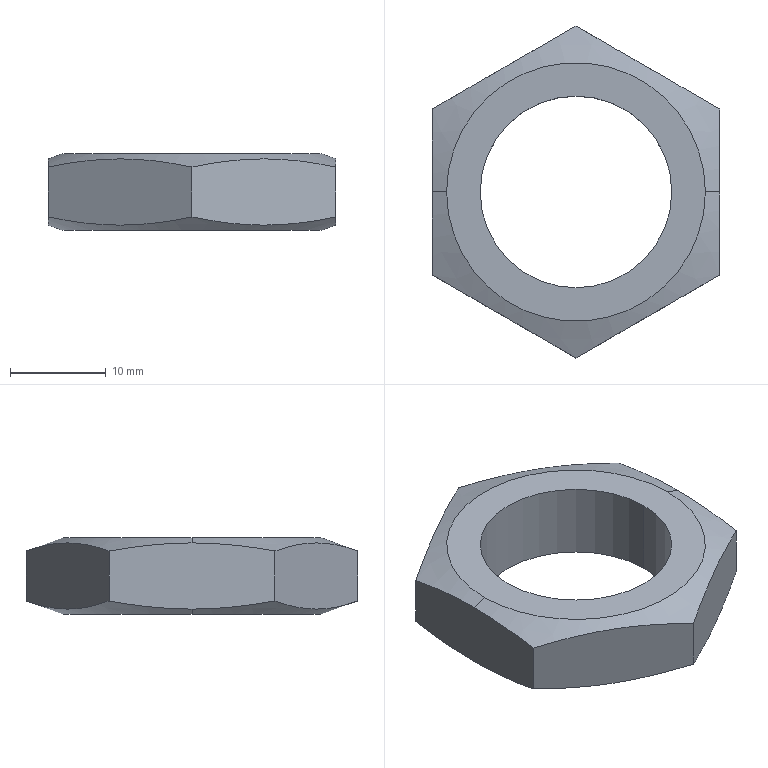Part | SolidWorks | features Extrusion 1, ICE 1, MirrorPattern 1, RefAxis 1, RevCut 1 | 1 solid | 14 faces | box 30 x 34.641 x 8 mm | volume 3531 mm3 | plane 8 | cone 4 | cylinder 2 | commonest cylinder face diameters 20 x2
STEP:
#1=CARTESIAN_POINT('',(-10.,0.,0.));
#2=VERTEX_POINT('',#1);
#3=CARTESIAN_POINT('',(10.,0.,0.));
#4=VERTEX_POINT('',#3);
#5=CARTESIAN_POINT('',(0.,0.,0.));
#6=DIRECTION('',(0.,0.,1.));
#7=DIRECTION('',(1.,0.,0.));
#8=AXIS2_PLACEMENT_3D('',#5,#6,#7);
#9=CIRCLE('',#8,10.);
#10=EDGE_CURVE('',#2,#4,#9,.T.);
#11=ORIENTED_EDGE('',*,*,#10,.F.);
#12=CARTESIAN_POINT('',(-10.,0.,8.));
#13=VERTEX_POINT('',#12);
#14=CARTESIAN_POINT('',(-10.,0.,0.));
#15=DIRECTION('',(0.,0.,1.));
#16=VECTOR('',#15,1000.);
#17=LINE('',#14,#16);
#18=EDGE_CURVE('',#2,#13,#17,.T.);
#19=ORIENTED_EDGE('',*,*,#18,.T.);
#20=CARTESIAN_POINT('',(10.,0.,8.));
#21=VERTEX_POINT('',#20);
#22=CARTESIAN_POINT('',(0.,0.,8.));
#23=DIRECTION('',(0.,0.,1.));
#24=DIRECTION('',(1.,0.,0.));
#25=AXIS2_PLACEMENT_3D('',#22,#23,#24);
#26=CIRCLE('',#25,10.);
#27=EDGE_CURVE('',#13,#21,#26,.T.);
#28=ORIENTED_EDGE('',*,*,#27,.T.);
#29=CARTESIAN_POINT('',(10.,0.,0.));
#30=DIRECTION('',(0.,0.,1.));
#31=VECTOR('',#30,1000.);
#32=LINE('',#29,#31);
#33=EDGE_CURVE('',#4,#21,#32,.T.);
#34=ORIENTED_EDGE('',*,*,#33,.F.);
#35=EDGE_LOOP('',(#11,#19,#28,#34));
#36=FACE_OUTER_BOUND('',#35,.T.);
#37=CARTESIAN_POINT('',(0.,0.,0.));
#38=DIRECTION('',(0.,0.,1.));
#39=DIRECTION('',(1.,0.,0.));
#40=AXIS2_PLACEMENT_3D('',#37,#38,#39);
#41=CYLINDRICAL_SURFACE('',#40,10.);
#42=ADVANCED_FACE('',(#36),#41,.F.);
#43=CARTESIAN_POINT('',(-13.5,0.,0.));
#44=VERTEX_POINT('',#43);
#45=CARTESIAN_POINT('',(13.5,0.,0.));
#46=VERTEX_POINT('',#45);
#47=CARTESIAN_POINT('',(0.,0.,0.));
#48=DIRECTION('',(0.,0.,1.));
#49=DIRECTION('',(1.,0.,0.));
#50=AXIS2_PLACEMENT_3D('',#47,#48,#49);
#51=CIRCLE('',#50,13.5);
#52=EDGE_CURVE('',#44,#46,#51,.T.);
#53=ORIENTED_EDGE('',*,*,#52,.T.);
#54=CARTESIAN_POINT('',(15.,0.,0.546));
#55=VERTEX_POINT('',#54);
#56=CARTESIAN_POINT('',(17.321,0.,1.391));
#57=DIRECTION('',(0.9397,0.,0.342));
#58=VECTOR('',#57,1000.);
#59=LINE('',#56,#58);
#60=EDGE_CURVE('',#46,#55,#59,.T.);
#61=ORIENTED_EDGE('',*,*,#60,.T.);
#62=CARTESIAN_POINT('',(15.,-8.66,1.391));
#63=VERTEX_POINT('',#62);
#64=CARTESIAN_POINT('',(15.,-8.66,1.391));
#65=CARTESIAN_POINT('',(15.,-7.226,1.13));
#66=CARTESIAN_POINT('',(15.,-5.777,0.915));
#67=CARTESIAN_POINT('',(15.,-2.886,0.6231));
#68=CARTESIAN_POINT('',(15.,-1.442,0.546));
#69=CARTESIAN_POINT('',(15.,0.,0.546));
#70=B_SPLINE_CURVE_WITH_KNOTS('',3,(#64,#65,#66,#67,#68,#69),.UNSPECIFIED.,.F.,.F.,(4,2,4),(0.01468,0.01904,0.02341),.UNSPECIFIED.);
#71=EDGE_CURVE('',#63,#55,#70,.T.);
#72=ORIENTED_EDGE('',*,*,#71,.F.);
#73=CARTESIAN_POINT('',(0.,-17.321,1.391));
#74=VERTEX_POINT('',#73);
#75=CARTESIAN_POINT('',(0.,-17.321,1.391));
#76=CARTESIAN_POINT('',(1.25,-16.599,1.128));
#77=CARTESIAN_POINT('',(2.5,-15.877,0.9146));
#78=CARTESIAN_POINT('',(5.,-14.434,0.6232));
#79=CARTESIAN_POINT('',(7.5,-12.99,0.4687));
#80=CARTESIAN_POINT('',(10.,-11.547,0.6232));
#81=CARTESIAN_POINT('',(12.5,-10.104,0.9146));
#82=CARTESIAN_POINT('',(13.75,-9.382,1.128));
#83=CARTESIAN_POINT('',(15.,-8.66,1.391));
#84=B_SPLINE_CURVE_WITH_KNOTS('',3,(#75,#76,#77,#78,#79,#80,#81,#82,#83),.UNSPECIFIED.,.F.,.F.,(4,2,1,2,4),(0.000000231,0.00433,0.00866,0.01299,0.01732),.UNSPECIFIED.);
#85=EDGE_CURVE('',#74,#63,#84,.T.);
#86=ORIENTED_EDGE('',*,*,#85,.F.);
#87=CARTESIAN_POINT('',(-15.,-8.66,1.391));
#88=VERTEX_POINT('',#87);
#89=CARTESIAN_POINT('',(-15.,-8.66,1.391));
#90=CARTESIAN_POINT('',(-13.75,-9.382,1.128));
#91=CARTESIAN_POINT('',(-12.5,-10.104,0.9146));
#92=CARTESIAN_POINT('',(-10.,-11.547,0.6232));
#93=CARTESIAN_POINT('',(-7.5,-12.99,0.4687));
#94=CARTESIAN_POINT('',(-5.,-14.434,0.6232));
#95=CARTESIAN_POINT('',(-2.5,-15.877,0.9146));
#96=CARTESIAN_POINT('',(-1.25,-16.599,1.128));
#97=CARTESIAN_POINT('',(0.,-17.321,1.391));
#98=B_SPLINE_CURVE_WITH_KNOTS('',3,(#89,#90,#91,#92,#93,#94,#95,#96,#97),.UNSPECIFIED.,.F.,.F.,(4,2,1,2,4),(0.000000231,0.00433,0.00866,0.01299,0.01732),.UNSPECIFIED.);
#99=EDGE_CURVE('',#88,#74,#98,.T.);
#100=ORIENTED_EDGE('',*,*,#99,.F.);
#101=CARTESIAN_POINT('',(-15.,0.,0.546));
#102=VERTEX_POINT('',#101);
#103=CARTESIAN_POINT('',(-15.,0.,0.546));
#104=CARTESIAN_POINT('',(-15.,-1.442,0.546));
#105=CARTESIAN_POINT('',(-15.,-2.886,0.6231));
#106=CARTESIAN_POINT('',(-15.,-5.777,0.915));
#107=CARTESIAN_POINT('',(-15.,-7.226,1.13));
#108=CARTESIAN_POINT('',(-15.,-8.66,1.391));
#109=B_SPLINE_CURVE_WITH_KNOTS('',3,(#103,#104,#105,#106,#107,#108),.UNSPECIFIED.,.F.,.F.,(4,2,4),(0.04016,0.04451,0.04886),.UNSPECIFIED.);
#110=EDGE_CURVE('',#102,#88,#109,.T.);
#111=ORIENTED_EDGE('',*,*,#110,.F.);
#112=CARTESIAN_POINT('',(-17.321,0.,1.391));
#113=DIRECTION('',(-0.9397,0.,0.342));
#114=VECTOR('',#113,1000.);
#115=LINE('',#112,#114);
#116=EDGE_CURVE('',#44,#102,#115,.T.);
#117=ORIENTED_EDGE('',*,*,#116,.F.);
#118=EDGE_LOOP('',(#53,#61,#72,#86,#100,#111,#117));
#119=FACE_OUTER_BOUND('',#118,.T.);
#120=CARTESIAN_POINT('',(0.,0.,1.391));
#121=DIRECTION('',(0.,0.,1.));
#122=DIRECTION('',(-1.,0.,0.));
#123=AXIS2_PLACEMENT_3D('',#120,#121,#122);
#124=CONICAL_SURFACE('',#123,17.321,1.222);
#125=ADVANCED_FACE('',(#119),#124,.T.);
#126=CARTESIAN_POINT('',(13.5,0.,8.));
#127=VERTEX_POINT('',#126);
#128=CARTESIAN_POINT('',(-13.5,0.,8.));
#129=VERTEX_POINT('',#128);
#130=CARTESIAN_POINT('',(0.,0.,8.));
#131=DIRECTION('',(0.,0.,1.));
#132=DIRECTION('',(1.,0.,0.));
#133=AXIS2_PLACEMENT_3D('',#130,#131,#132);
#134=CIRCLE('',#133,13.5);
#135=EDGE_CURVE('',#127,#129,#134,.T.);
#136=ORIENTED_EDGE('',*,*,#135,.F.);
#137=CARTESIAN_POINT('',(15.,0.,7.454));
#138=VERTEX_POINT('',#137);
#139=CARTESIAN_POINT('',(17.321,0.,6.609));
#140=DIRECTION('',(0.9397,0.,-0.342));
#141=VECTOR('',#140,1000.);
#142=LINE('',#139,#141);
#143=EDGE_CURVE('',#127,#138,#142,.T.);
#144=ORIENTED_EDGE('',*,*,#143,.T.);
#145=CARTESIAN_POINT('',(15.,8.66,6.609));
#146=VERTEX_POINT('',#145);
#147=CARTESIAN_POINT('',(15.,8.66,6.609));
#148=CARTESIAN_POINT('',(15.,7.221,6.871));
#149=CARTESIAN_POINT('',(15.,5.778,7.085));
#150=CARTESIAN_POINT('',(15.,2.891,7.377));
#151=CARTESIAN_POINT('',(15.,1.446,7.454));
#152=CARTESIAN_POINT('',(15.,0.,7.454));
#153=B_SPLINE_CURVE_WITH_KNOTS('',3,(#147,#148,#149,#150,#151,#152),.UNSPECIFIED.,.F.,.F.,(4,2,4),(0.03143,0.03579,0.04016),.UNSPECIFIED.);
#154=EDGE_CURVE('',#146,#138,#153,.T.);
#155=ORIENTED_EDGE('',*,*,#154,.F.);
#156=CARTESIAN_POINT('',(0.,17.321,6.609));
#157=VERTEX_POINT('',#156);
#158=CARTESIAN_POINT('',(0.,17.321,6.609));
#159=CARTESIAN_POINT('',(1.25,16.599,6.872));
#160=CARTESIAN_POINT('',(2.5,15.877,7.085));
#161=CARTESIAN_POINT('',(5.,14.434,7.377));
#162=CARTESIAN_POINT('',(7.5,12.99,7.531));
#163=CARTESIAN_POINT('',(10.,11.547,7.377));
#164=CARTESIAN_POINT('',(12.5,10.104,7.085));
#165=CARTESIAN_POINT('',(13.75,9.382,6.872));
#166=CARTESIAN_POINT('',(15.,8.66,6.609));
#167=B_SPLINE_CURVE_WITH_KNOTS('',3,(#158,#159,#160,#161,#162,#163,#164,#165,#166),.UNSPECIFIED.,.F.,.F.,(4,2,1,2,4),(0.000000231,0.00433,0.00866,0.01299,0.01732),.UNSPECIFIED.);
#168=EDGE_CURVE('',#157,#146,#167,.T.);
#169=ORIENTED_EDGE('',*,*,#168,.F.);
#170=CARTESIAN_POINT('',(-15.,8.66,6.609));
#171=VERTEX_POINT('',#170);
#172=CARTESIAN_POINT('',(-15.,8.66,6.609));
#173=CARTESIAN_POINT('',(-13.75,9.382,6.872));
#174=CARTESIAN_POINT('',(-12.5,10.104,7.085));
#175=CARTESIAN_POINT('',(-10.,11.547,7.377));
#176=CARTESIAN_POINT('',(-7.5,12.99,7.531));
#177=CARTESIAN_POINT('',(-5.,14.434,7.377));
#178=CARTESIAN_POINT('',(-2.5,15.877,7.085));
#179=CARTESIAN_POINT('',(-1.25,16.599,6.872));
#180=CARTESIAN_POINT('',(0.,17.321,6.609));
#181=B_SPLINE_CURVE_WITH_KNOTS('',3,(#172,#173,#174,#175,#176,#177,#178,#179,#180),.UNSPECIFIED.,.F.,.F.,(4,2,1,2,4),(0.000000231,0.00433,0.00866,0.01299,0.01732),.UNSPECIFIED.);
#182=EDGE_CURVE('',#171,#157,#181,.T.);
#183=ORIENTED_EDGE('',*,*,#182,.F.);
#184=CARTESIAN_POINT('',(-15.,0.,7.454));
#185=VERTEX_POINT('',#184);
#186=CARTESIAN_POINT('',(-15.,0.,7.454));
#187=CARTESIAN_POINT('',(-15.,1.446,7.454));
#188=CARTESIAN_POINT('',(-15.,2.891,7.377));
#189=CARTESIAN_POINT('',(-15.,5.778,7.085));
#190=CARTESIAN_POINT('',(-15.,7.221,6.871));
#191=CARTESIAN_POINT('',(-15.,8.66,6.609));
#192=B_SPLINE_CURVE_WITH_KNOTS('',3,(#186,#187,#188,#189,#190,#191),.UNSPECIFIED.,.F.,.F.,(4,2,4),(0.02341,0.02778,0.03216),.UNSPECIFIED.);
#193=EDGE_CURVE('',#185,#171,#192,.T.);
#194=ORIENTED_EDGE('',*,*,#193,.F.);
#195=CARTESIAN_POINT('',(-17.321,0.,6.609));
#196=DIRECTION('',(-0.9397,0.,-0.342));
#197=VECTOR('',#196,1000.);
#198=LINE('',#195,#197);
#199=EDGE_CURVE('',#129,#185,#198,.T.);
#200=ORIENTED_EDGE('',*,*,#199,.F.);
#201=EDGE_LOOP('',(#136,#144,#155,#169,#183,#194,#200));
#202=FACE_OUTER_BOUND('',#201,.T.);
#203=CARTESIAN_POINT('',(0.,0.,6.609));
#204=DIRECTION('',(0.,0.,-1.));
#205=DIRECTION('',(-1.,0.,0.));
#206=AXIS2_PLACEMENT_3D('',#203,#204,#205);
#207=CONICAL_SURFACE('',#206,17.321,1.222);
#208=ADVANCED_FACE('',(#202),#207,.T.);
#209=CARTESIAN_POINT('',(15.,8.66,1.391));
#210=VERTEX_POINT('',#209);
#211=CARTESIAN_POINT('',(15.,8.66,8.));
#212=DIRECTION('',(0.,0.,-1.));
#213=VECTOR('',#212,1000.);
#214=LINE('',#211,#213);
#215=EDGE_CURVE('',#146,#210,#214,.T.);
#216=ORIENTED_EDGE('',*,*,#215,.T.);
#217=CARTESIAN_POINT('',(0.,17.321,1.391));
#218=VERTEX_POINT('',#217);
#219=CARTESIAN_POINT('',(15.,8.66,1.391));
#220=CARTESIAN_POINT('',(13.75,9.382,1.128));
#221=CARTESIAN_POINT('',(12.5,10.104,0.9146));
#222=CARTESIAN_POINT('',(10.,11.547,0.6232));
#223=CARTESIAN_POINT('',(7.5,12.99,0.4687));
#224=CARTESIAN_POINT('',(5.,14.434,0.6232));
#225=CARTESIAN_POINT('',(2.5,15.877,0.9146));
#226=CARTESIAN_POINT('',(1.25,16.599,1.128));
#227=CARTESIAN_POINT('',(0.,17.321,1.391));
#228=B_SPLINE_CURVE_WITH_KNOTS('',3,(#219,#220,#221,#222,#223,#224,#225,#226,#227),.UNSPECIFIED.,.F.,.F.,(4,2,1,2,4),(0.000000231,0.00433,0.00866,0.01299,0.01732),.UNSPECIFIED.);
#229=EDGE_CURVE('',#210,#218,#228,.T.);
#230=ORIENTED_EDGE('',*,*,#229,.T.);
#231=CARTESIAN_POINT('',(0.,17.321,8.));
#232=DIRECTION('',(0.,0.,-1.));
#233=VECTOR('',#232,1000.);
#234=LINE('',#231,#233);
#235=EDGE_CURVE('',#157,#218,#234,.T.);
#236=ORIENTED_EDGE('',*,*,#235,.F.);
#237=ORIENTED_EDGE('',*,*,#168,.T.);
#238=EDGE_LOOP('',(#216,#230,#236,#237));
#239=FACE_OUTER_BOUND('',#238,.T.);
#240=CARTESIAN_POINT('',(15.,8.66,8.));
#241=DIRECTION('',(-0.5,-0.866,0.));
#242=DIRECTION('',(0.866,-0.5,0.));
#243=AXIS2_PLACEMENT_3D('',#240,#241,#242);
#244=PLANE('',#243);
#245=ADVANCED_FACE('',(#239),#244,.F.);
#246=ORIENTED_EDGE('',*,*,#235,.T.);
#247=CARTESIAN_POINT('',(-15.,8.66,1.391));
#248=VERTEX_POINT('',#247);
#249=CARTESIAN_POINT('',(0.,17.321,1.391));
#250=CARTESIAN_POINT('',(-1.25,16.599,1.128));
#251=CARTESIAN_POINT('',(-2.5,15.877,0.9146));
#252=CARTESIAN_POINT('',(-5.,14.434,0.6232));
#253=CARTESIAN_POINT('',(-7.5,12.99,0.4687));
#254=CARTESIAN_POINT('',(-10.,11.547,0.6232));
#255=CARTESIAN_POINT('',(-12.5,10.104,0.9146));
#256=CARTESIAN_POINT('',(-13.75,9.382,1.128));
#257=CARTESIAN_POINT('',(-15.,8.66,1.391));
#258=B_SPLINE_CURVE_WITH_KNOTS('',3,(#249,#250,#251,#252,#253,#254,#255,#256,#257),.UNSPECIFIED.,.F.,.F.,(4,2,1,2,4),(0.000000231,0.00433,0.00866,0.01299,0.01732),.UNSPECIFIED.);
#259=EDGE_CURVE('',#218,#248,#258,.T.);
#260=ORIENTED_EDGE('',*,*,#259,.T.);
#261=CARTESIAN_POINT('',(-15.,8.66,8.));
#262=DIRECTION('',(0.,0.,-1.));
#263=VECTOR('',#262,1000.);
#264=LINE('',#261,#263);
#265=EDGE_CURVE('',#171,#248,#264,.T.);
#266=ORIENTED_EDGE('',*,*,#265,.F.);
#267=ORIENTED_EDGE('',*,*,#182,.T.);
#268=EDGE_LOOP('',(#246,#260,#266,#267));
#269=FACE_OUTER_BOUND('',#268,.T.);
#270=CARTESIAN_POINT('',(0.,17.321,8.));
#271=DIRECTION('',(0.5,-0.866,0.));
#272=DIRECTION('',(0.866,0.5,0.));
#273=AXIS2_PLACEMENT_3D('',#270,#271,#272);
#274=PLANE('',#273);
#275=ADVANCED_FACE('',(#269),#274,.F.);
#276=ORIENTED_EDGE('',*,*,#265,.T.);
#277=CARTESIAN_POINT('',(-15.,8.66,1.391));
#278=CARTESIAN_POINT('',(-15.,7.221,1.129));
#279=CARTESIAN_POINT('',(-15.,5.778,0.9152));
#280=CARTESIAN_POINT('',(-15.,2.891,0.6235));
#281=CARTESIAN_POINT('',(-15.,1.446,0.546));
#282=CARTESIAN_POINT('',(-15.,0.,0.546));
#283=B_SPLINE_CURVE_WITH_KNOTS('',3,(#277,#278,#279,#280,#281,#282),.UNSPECIFIED.,.F.,.F.,(4,2,4),(0.03143,0.03579,0.04016),.UNSPECIFIED.);
#284=EDGE_CURVE('',#248,#102,#283,.T.);
#285=ORIENTED_EDGE('',*,*,#284,.T.);
#286=ORIENTED_EDGE('',*,*,#110,.T.);
#287=CARTESIAN_POINT('',(-15.,-8.66,6.609));
#288=VERTEX_POINT('',#287);
#289=CARTESIAN_POINT('',(-15.,-8.66,8.));
#290=DIRECTION('',(0.,0.,-1.));
#291=VECTOR('',#290,1000.);
#292=LINE('',#289,#291);
#293=EDGE_CURVE('',#288,#88,#292,.T.);
#294=ORIENTED_EDGE('',*,*,#293,.F.);
#295=CARTESIAN_POINT('',(-15.,-8.66,6.609));
#296=CARTESIAN_POINT('',(-15.,-7.226,6.87));
#297=CARTESIAN_POINT('',(-15.,-5.777,7.085));
#298=CARTESIAN_POINT('',(-15.,-2.886,7.377));
#299=CARTESIAN_POINT('',(-15.,-1.442,7.454));
#300=CARTESIAN_POINT('',(-15.,0.,7.454));
#301=B_SPLINE_CURVE_WITH_KNOTS('',3,(#295,#296,#297,#298,#299,#300),.UNSPECIFIED.,.F.,.F.,(4,2,4),(0.01468,0.01904,0.02341),.UNSPECIFIED.);
#302=EDGE_CURVE('',#288,#185,#301,.T.);
#303=ORIENTED_EDGE('',*,*,#302,.T.);
#304=ORIENTED_EDGE('',*,*,#193,.T.);
#305=EDGE_LOOP('',(#276,#285,#286,#294,#303,#304));
#306=FACE_OUTER_BOUND('',#305,.T.);
#307=CARTESIAN_POINT('',(-15.,8.66,8.));
#308=DIRECTION('',(1.,0.,0.));
#309=DIRECTION('',(0.,0.,-1.));
#310=AXIS2_PLACEMENT_3D('',#307,#308,#309);
#311=PLANE('',#310);
#312=ADVANCED_FACE('',(#306),#311,.F.);
#313=ORIENTED_EDGE('',*,*,#293,.T.);
#314=ORIENTED_EDGE('',*,*,#99,.T.);
#315=CARTESIAN_POINT('',(0.,-17.321,6.609));
#316=VERTEX_POINT('',#315);
#317=CARTESIAN_POINT('',(0.,-17.321,8.));
#318=DIRECTION('',(0.,0.,-1.));
#319=VECTOR('',#318,1000.);
#320=LINE('',#317,#319);
#321=EDGE_CURVE('',#316,#74,#320,.T.);
#322=ORIENTED_EDGE('',*,*,#321,.F.);
#323=CARTESIAN_POINT('',(0.,-17.321,6.609));
#324=CARTESIAN_POINT('',(-1.25,-16.599,6.872));
#325=CARTESIAN_POINT('',(-2.5,-15.877,7.085));
#326=CARTESIAN_POINT('',(-5.,-14.434,7.377));
#327=CARTESIAN_POINT('',(-7.5,-12.99,7.531));
#328=CARTESIAN_POINT('',(-10.,-11.547,7.377));
#329=CARTESIAN_POINT('',(-12.5,-10.104,7.085));
#330=CARTESIAN_POINT('',(-13.75,-9.382,6.872));
#331=CARTESIAN_POINT('',(-15.,-8.66,6.609));
#332=B_SPLINE_CURVE_WITH_KNOTS('',3,(#323,#324,#325,#326,#327,#328,#329,#330,#331),.UNSPECIFIED.,.F.,.F.,(4,2,1,2,4),(0.000000231,0.00433,0.00866,0.01299,0.01732),.UNSPECIFIED.);
#333=EDGE_CURVE('',#316,#288,#332,.T.);
#334=ORIENTED_EDGE('',*,*,#333,.T.);
#335=EDGE_LOOP('',(#313,#314,#322,#334));
#336=FACE_OUTER_BOUND('',#335,.T.);
#337=CARTESIAN_POINT('',(-15.,-8.66,8.));
#338=DIRECTION('',(0.5,0.866,0.));
#339=DIRECTION('',(-0.866,0.5,0.));
#340=AXIS2_PLACEMENT_3D('',#337,#338,#339);
#341=PLANE('',#340);
#342=ADVANCED_FACE('',(#336),#341,.F.);
#343=ORIENTED_EDGE('',*,*,#321,.T.);
#344=ORIENTED_EDGE('',*,*,#85,.T.);
#345=CARTESIAN_POINT('',(15.,-8.66,6.609));
#346=VERTEX_POINT('',#345);
#347=CARTESIAN_POINT('',(15.,-8.66,8.));
#348=DIRECTION('',(0.,0.,-1.));
#349=VECTOR('',#348,1000.);
#350=LINE('',#347,#349);
#351=EDGE_CURVE('',#346,#63,#350,.T.);
#352=ORIENTED_EDGE('',*,*,#351,.F.);
#353=CARTESIAN_POINT('',(15.,-8.66,6.609));
#354=CARTESIAN_POINT('',(13.75,-9.382,6.872));
#355=CARTESIAN_POINT('',(12.5,-10.104,7.085));
#356=CARTESIAN_POINT('',(10.,-11.547,7.377));
#357=CARTESIAN_POINT('',(7.5,-12.99,7.531));
#358=CARTESIAN_POINT('',(5.,-14.434,7.377));
#359=CARTESIAN_POINT('',(2.5,-15.877,7.085));
#360=CARTESIAN_POINT('',(1.25,-16.599,6.872));
#361=CARTESIAN_POINT('',(0.,-17.321,6.609));
#362=B_SPLINE_CURVE_WITH_KNOTS('',3,(#353,#354,#355,#356,#357,#358,#359,#360,#361),.UNSPECIFIED.,.F.,.F.,(4,2,1,2,4),(0.000000231,0.00433,0.00866,0.01299,0.01732),.UNSPECIFIED.);
#363=EDGE_CURVE('',#346,#316,#362,.T.);
#364=ORIENTED_EDGE('',*,*,#363,.T.);
#365=EDGE_LOOP('',(#343,#344,#352,#364));
#366=FACE_OUTER_BOUND('',#365,.T.);
#367=CARTESIAN_POINT('',(0.,-17.321,8.));
#368=DIRECTION('',(-0.5,0.866,0.));
#369=DIRECTION('',(-0.866,-0.5,0.));
#370=AXIS2_PLACEMENT_3D('',#367,#368,#369);
#371=PLANE('',#370);
#372=ADVANCED_FACE('',(#366),#371,.F.);
#373=ORIENTED_EDGE('',*,*,#351,.T.);
#374=ORIENTED_EDGE('',*,*,#71,.T.);
#375=CARTESIAN_POINT('',(15.,0.,0.546));
#376=CARTESIAN_POINT('',(15.,1.446,0.546));
#377=CARTESIAN_POINT('',(15.,2.891,0.6235));
#378=CARTESIAN_POINT('',(15.,5.778,0.9152));
#379=CARTESIAN_POINT('',(15.,7.221,1.129));
#380=CARTESIAN_POINT('',(15.,8.66,1.391));
#381=B_SPLINE_CURVE_WITH_KNOTS('',3,(#375,#376,#377,#378,#379,#380),.UNSPECIFIED.,.F.,.F.,(4,2,4),(0.02341,0.02778,0.03216),.UNSPECIFIED.);
#382=EDGE_CURVE('',#55,#210,#381,.T.);
#383=ORIENTED_EDGE('',*,*,#382,.T.);
#384=ORIENTED_EDGE('',*,*,#215,.F.);
#385=ORIENTED_EDGE('',*,*,#154,.T.);
#386=CARTESIAN_POINT('',(15.,0.,7.454));
#387=CARTESIAN_POINT('',(15.,-1.442,7.454));
#388=CARTESIAN_POINT('',(15.,-2.886,7.377));
#389=CARTESIAN_POINT('',(15.,-5.777,7.085));
#390=CARTESIAN_POINT('',(15.,-7.226,6.87));
#391=CARTESIAN_POINT('',(15.,-8.66,6.609));
#392=B_SPLINE_CURVE_WITH_KNOTS('',3,(#386,#387,#388,#389,#390,#391),.UNSPECIFIED.,.F.,.F.,(4,2,4),(0.04016,0.04451,0.04886),.UNSPECIFIED.);
#393=EDGE_CURVE('',#138,#346,#392,.T.);
#394=ORIENTED_EDGE('',*,*,#393,.T.);
#395=EDGE_LOOP('',(#373,#374,#383,#384,#385,#394));
#396=FACE_OUTER_BOUND('',#395,.T.);
#397=CARTESIAN_POINT('',(15.,-8.66,8.));
#398=DIRECTION('',(-1.,0.,0.));
#399=DIRECTION('',(0.,-1.,0.));
#400=AXIS2_PLACEMENT_3D('',#397,#398,#399);
#401=PLANE('',#400);
#402=ADVANCED_FACE('',(#396),#401,.F.);
#403=ORIENTED_EDGE('',*,*,#143,.F.);
#404=CARTESIAN_POINT('',(0.,0.,8.));
#405=DIRECTION('',(0.,0.,1.));
#406=DIRECTION('',(1.,0.,0.));
#407=AXIS2_PLACEMENT_3D('',#404,#405,#406);
#408=CIRCLE('',#407,13.5);
#409=EDGE_CURVE('',#129,#127,#408,.T.);
#410=ORIENTED_EDGE('',*,*,#409,.F.);
#411=ORIENTED_EDGE('',*,*,#199,.T.);
#412=ORIENTED_EDGE('',*,*,#302,.F.);
#413=ORIENTED_EDGE('',*,*,#333,.F.);
#414=ORIENTED_EDGE('',*,*,#363,.F.);
#415=ORIENTED_EDGE('',*,*,#393,.F.);
#416=EDGE_LOOP('',(#403,#410,#411,#412,#413,#414,#415));
#417=FACE_OUTER_BOUND('',#416,.T.);
#418=CARTESIAN_POINT('',(0.,0.,6.609));
#419=DIRECTION('',(0.,0.,-1.));
#420=DIRECTION('',(-1.,0.,0.));
#421=AXIS2_PLACEMENT_3D('',#418,#419,#420);
#422=CONICAL_SURFACE('',#421,17.321,1.222);
#423=ADVANCED_FACE('',(#417),#422,.T.);
#424=CARTESIAN_POINT('',(0.,0.,8.));
#425=DIRECTION('',(0.,0.,1.));
#426=DIRECTION('',(1.,0.,0.));
#427=AXIS2_PLACEMENT_3D('',#424,#425,#426);
#428=CIRCLE('',#427,10.);
#429=EDGE_CURVE('',#21,#13,#428,.T.);
#430=ORIENTED_EDGE('',*,*,#429,.F.);
#431=ORIENTED_EDGE('',*,*,#27,.F.);
#432=EDGE_LOOP('',(#430,#431));
#433=FACE_BOUND('',#432,.T.);
#434=ORIENTED_EDGE('',*,*,#409,.T.);
#435=ORIENTED_EDGE('',*,*,#135,.T.);
#436=EDGE_LOOP('',(#434,#435));
#437=FACE_OUTER_BOUND('',#436,.T.);
#438=CARTESIAN_POINT('',(0.,0.,8.));
#439=DIRECTION('',(0.,0.,1.));
#440=DIRECTION('',(1.,0.,0.));
#441=AXIS2_PLACEMENT_3D('',#438,#439,#440);
#442=PLANE('',#441);
#443=ADVANCED_FACE('',(#433,#437),#442,.T.);
#444=ORIENTED_EDGE('',*,*,#60,.F.);
#445=CARTESIAN_POINT('',(0.,0.,0.));
#446=DIRECTION('',(0.,0.,1.));
#447=DIRECTION('',(1.,0.,0.));
#448=AXIS2_PLACEMENT_3D('',#445,#446,#447);
#449=CIRCLE('',#448,13.5);
#450=EDGE_CURVE('',#46,#44,#449,.T.);
#451=ORIENTED_EDGE('',*,*,#450,.T.);
#452=ORIENTED_EDGE('',*,*,#116,.T.);
#453=ORIENTED_EDGE('',*,*,#284,.F.);
#454=ORIENTED_EDGE('',*,*,#259,.F.);
#455=ORIENTED_EDGE('',*,*,#229,.F.);
#456=ORIENTED_EDGE('',*,*,#382,.F.);
#457=EDGE_LOOP('',(#444,#451,#452,#453,#454,#455,#456));
#458=FACE_OUTER_BOUND('',#457,.T.);
#459=CARTESIAN_POINT('',(0.,0.,1.391));
#460=DIRECTION('',(0.,0.,1.));
#461=DIRECTION('',(-1.,0.,0.));
#462=AXIS2_PLACEMENT_3D('',#459,#460,#461);
#463=CONICAL_SURFACE('',#462,17.321,1.222);
#464=ADVANCED_FACE('',(#458),#463,.T.);
#465=CARTESIAN_POINT('',(0.,0.,0.));
#466=DIRECTION('',(0.,0.,1.));
#467=DIRECTION('',(1.,0.,0.));
#468=AXIS2_PLACEMENT_3D('',#465,#466,#467);
#469=CIRCLE('',#468,10.);
#470=EDGE_CURVE('',#4,#2,#469,.T.);
#471=ORIENTED_EDGE('',*,*,#470,.T.);
#472=ORIENTED_EDGE('',*,*,#10,.T.);
#473=EDGE_LOOP('',(#471,#472));
#474=FACE_BOUND('',#473,.T.);
#475=ORIENTED_EDGE('',*,*,#52,.F.);
#476=ORIENTED_EDGE('',*,*,#450,.F.);
#477=EDGE_LOOP('',(#475,#476));
#478=FACE_OUTER_BOUND('',#477,.T.);
#479=CARTESIAN_POINT('',(0.,0.,0.));
#480=DIRECTION('',(0.,0.,1.));
#481=DIRECTION('',(1.,0.,0.));
#482=AXIS2_PLACEMENT_3D('',#479,#480,#481);
#483=PLANE('',#482);
#484=ADVANCED_FACE('',(#474,#478),#483,.F.);
#485=ORIENTED_EDGE('',*,*,#18,.F.);
#486=ORIENTED_EDGE('',*,*,#470,.F.);
#487=ORIENTED_EDGE('',*,*,#33,.T.);
#488=ORIENTED_EDGE('',*,*,#429,.T.);
#489=EDGE_LOOP('',(#485,#486,#487,#488));
#490=FACE_OUTER_BOUND('',#489,.T.);
#491=CARTESIAN_POINT('',(0.,0.,0.));
#492=DIRECTION('',(0.,0.,1.));
#493=DIRECTION('',(1.,0.,0.));
#494=AXIS2_PLACEMENT_3D('',#491,#492,#493);
#495=CYLINDRICAL_SURFACE('',#494,10.);
#496=ADVANCED_FACE('',(#490),#495,.F.);
#497=CLOSED_SHELL('',(#42,#125,#208,#245,#275,#312,#342,#372,#402,#423,#443,#464,#484,#496));
#498=MANIFOLD_SOLID_BREP('',#497);
#499=CARTESIAN_POINT('',(0.,0.,0.));
#500=DIRECTION('',(0.,0.,1.));
#501=DIRECTION('',(1.,0.,0.));
#502=AXIS2_PLACEMENT_3D('',#499,#500,#501);
#503=(LENGTH_UNIT()NAMED_UNIT(*)SI_UNIT(.MILLI.,.METRE.));
#504=UNCERTAINTY_MEASURE_WITH_UNIT(LENGTH_MEASURE(0.00001),#503,'','');
#505=(NAMED_UNIT(*)PLANE_ANGLE_UNIT()SI_UNIT($,.RADIAN.));
#506=(NAMED_UNIT(*)SI_UNIT($,.STERADIAN.)SOLID_ANGLE_UNIT());
#507=(GEOMETRIC_REPRESENTATION_CONTEXT(3)GLOBAL_UNCERTAINTY_ASSIGNED_CONTEXT((#504))GLOBAL_UNIT_ASSIGNED_CONTEXT((#503,#505,#506))REPRESENTATION_CONTEXT('',''));
#508=ADVANCED_BREP_SHAPE_REPRESENTATION('',(#498,#502),#507);